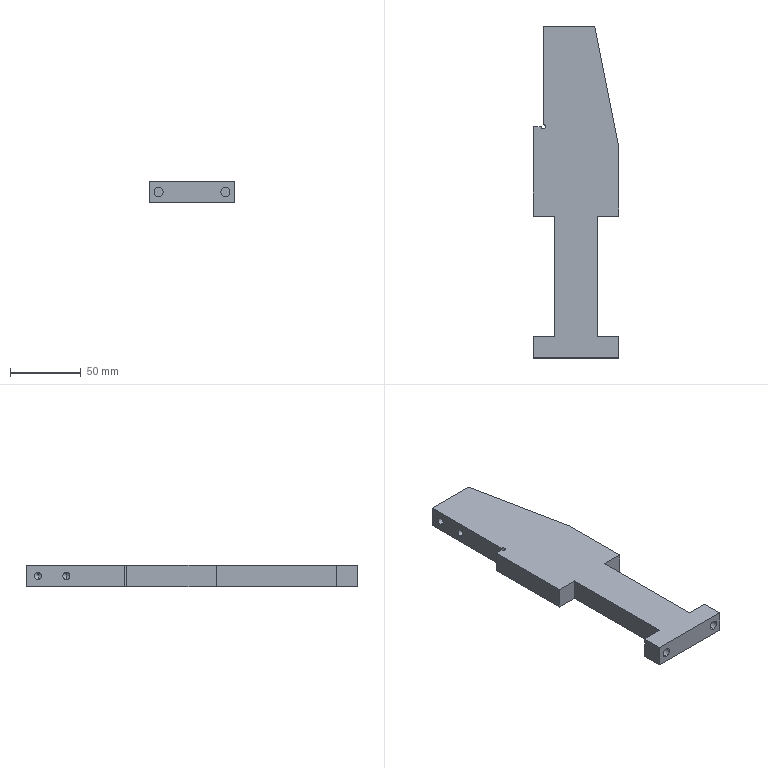Part | STEP file | 11-FG-E00211 | 1 solid | 31 faces | box 60 x 234 x 15 mm | volume 152627 mm3 | plane 17 | cylinder 10 | cone 4 | commonest cylinder face diameters 5 x4 6.5 x4 3 x2
STEP:
#1=CARTESIAN_POINT('',(6.5,0.,4.25));
#2=VERTEX_POINT('',#1);
#3=CARTESIAN_POINT('',(6.5,0.,10.75));
#4=VERTEX_POINT('',#3);
#5=CARTESIAN_POINT('',(6.5,0.,7.5));
#6=DIRECTION('',(0.,1.,0.));
#7=DIRECTION('',(0.,0.,1.));
#8=AXIS2_PLACEMENT_3D('',#5,#6,#7);
#9=CIRCLE('',#8,3.25);
#10=EDGE_CURVE('',#2,#4,#9,.T.);
#11=ORIENTED_EDGE('',*,*,#10,.F.);
#12=CARTESIAN_POINT('',(6.5,15.,4.25));
#13=VERTEX_POINT('',#12);
#14=CARTESIAN_POINT('',(6.5,-46.,4.25));
#15=DIRECTION('',(0.,1.,0.));
#16=VECTOR('',#15,1000.);
#17=LINE('',#14,#16);
#18=EDGE_CURVE('',#2,#13,#17,.T.);
#19=ORIENTED_EDGE('',*,*,#18,.T.);
#20=CARTESIAN_POINT('',(6.5,15.,10.75));
#21=VERTEX_POINT('',#20);
#22=CARTESIAN_POINT('',(6.5,15.,7.5));
#23=DIRECTION('',(0.,1.,0.));
#24=DIRECTION('',(0.,0.,1.));
#25=AXIS2_PLACEMENT_3D('',#22,#23,#24);
#26=CIRCLE('',#25,3.25);
#27=EDGE_CURVE('',#13,#21,#26,.T.);
#28=ORIENTED_EDGE('',*,*,#27,.T.);
#29=CARTESIAN_POINT('',(6.5,-46.,10.75));
#30=DIRECTION('',(0.,1.,0.));
#31=VECTOR('',#30,1000.);
#32=LINE('',#29,#31);
#33=EDGE_CURVE('',#4,#21,#32,.T.);
#34=ORIENTED_EDGE('',*,*,#33,.F.);
#35=EDGE_LOOP('',(#11,#19,#28,#34));
#36=FACE_OUTER_BOUND('',#35,.T.);
#37=CARTESIAN_POINT('',(6.5,-46.,7.5));
#38=DIRECTION('',(0.,1.,0.));
#39=DIRECTION('',(0.,0.,1.));
#40=AXIS2_PLACEMENT_3D('',#37,#38,#39);
#41=CYLINDRICAL_SURFACE('',#40,3.25);
#42=ADVANCED_FACE('',(#36),#41,.F.);
#43=CARTESIAN_POINT('',(53.5,0.,4.25));
#44=VERTEX_POINT('',#43);
#45=CARTESIAN_POINT('',(53.5,0.,10.75));
#46=VERTEX_POINT('',#45);
#47=CARTESIAN_POINT('',(53.5,0.,7.5));
#48=DIRECTION('',(0.,1.,0.));
#49=DIRECTION('',(0.,0.,1.));
#50=AXIS2_PLACEMENT_3D('',#47,#48,#49);
#51=CIRCLE('',#50,3.25);
#52=EDGE_CURVE('',#44,#46,#51,.T.);
#53=ORIENTED_EDGE('',*,*,#52,.F.);
#54=CARTESIAN_POINT('',(53.5,15.,4.25));
#55=VERTEX_POINT('',#54);
#56=CARTESIAN_POINT('',(53.5,-46.,4.25));
#57=DIRECTION('',(0.,1.,0.));
#58=VECTOR('',#57,1000.);
#59=LINE('',#56,#58);
#60=EDGE_CURVE('',#44,#55,#59,.T.);
#61=ORIENTED_EDGE('',*,*,#60,.T.);
#62=CARTESIAN_POINT('',(53.5,15.,10.75));
#63=VERTEX_POINT('',#62);
#64=CARTESIAN_POINT('',(53.5,15.,7.5));
#65=DIRECTION('',(0.,1.,0.));
#66=DIRECTION('',(0.,0.,1.));
#67=AXIS2_PLACEMENT_3D('',#64,#65,#66);
#68=CIRCLE('',#67,3.25);
#69=EDGE_CURVE('',#55,#63,#68,.T.);
#70=ORIENTED_EDGE('',*,*,#69,.T.);
#71=CARTESIAN_POINT('',(53.5,-46.,10.75));
#72=DIRECTION('',(0.,1.,0.));
#73=VECTOR('',#72,1000.);
#74=LINE('',#71,#73);
#75=EDGE_CURVE('',#46,#63,#74,.T.);
#76=ORIENTED_EDGE('',*,*,#75,.F.);
#77=EDGE_LOOP('',(#53,#61,#70,#76));
#78=FACE_OUTER_BOUND('',#77,.T.);
#79=CARTESIAN_POINT('',(53.5,-46.,7.5));
#80=DIRECTION('',(0.,1.,0.));
#81=DIRECTION('',(0.,0.,1.));
#82=AXIS2_PLACEMENT_3D('',#79,#80,#81);
#83=CYLINDRICAL_SURFACE('',#82,3.25);
#84=ADVANCED_FACE('',(#78),#83,.F.);
#85=CARTESIAN_POINT('',(23.502,205.5,7.5));
#86=VERTEX_POINT('',#85);
#87=CARTESIAN_POINT('',(22.,205.5,10.));
#88=VERTEX_POINT('',#87);
#89=CARTESIAN_POINT('',(22.,205.5,10.));
#90=DIRECTION('',(-0.515,0.,0.8572));
#91=VECTOR('',#90,1000.);
#92=LINE('',#89,#91);
#93=EDGE_CURVE('',#86,#88,#92,.T.);
#94=ORIENTED_EDGE('',*,*,#93,.F.);
#95=CARTESIAN_POINT('',(22.,205.5,5.));
#96=VERTEX_POINT('',#95);
#97=CARTESIAN_POINT('',(22.,205.5,5.));
#98=DIRECTION('',(-0.515,0.,-0.8572));
#99=VECTOR('',#98,1000.);
#100=LINE('',#97,#99);
#101=EDGE_CURVE('',#86,#96,#100,.T.);
#102=ORIENTED_EDGE('',*,*,#101,.T.);
#103=CARTESIAN_POINT('',(22.,205.5,7.5));
#104=DIRECTION('',(-1.,0.,0.));
#105=DIRECTION('',(0.,0.,1.));
#106=AXIS2_PLACEMENT_3D('',#103,#104,#105);
#107=CIRCLE('',#106,2.5);
#108=EDGE_CURVE('',#96,#88,#107,.T.);
#109=ORIENTED_EDGE('',*,*,#108,.T.);
#110=EDGE_LOOP('',(#94,#102,#109));
#111=FACE_OUTER_BOUND('',#110,.T.);
#112=CARTESIAN_POINT('',(22.,205.5,7.5));
#113=DIRECTION('',(-1.,0.,0.));
#114=DIRECTION('',(0.,0.,1.));
#115=AXIS2_PLACEMENT_3D('',#112,#113,#114);
#116=CONICAL_SURFACE('',#115,2.5,1.03);
#117=ADVANCED_FACE('',(#111),#116,.F.);
#118=ORIENTED_EDGE('',*,*,#108,.F.);
#119=CARTESIAN_POINT('',(7.,205.5,5.));
#120=VERTEX_POINT('',#119);
#121=CARTESIAN_POINT('',(7.,205.5,5.));
#122=DIRECTION('',(-1.,0.,0.));
#123=VECTOR('',#122,1000.);
#124=LINE('',#121,#123);
#125=EDGE_CURVE('',#96,#120,#124,.T.);
#126=ORIENTED_EDGE('',*,*,#125,.T.);
#127=CARTESIAN_POINT('',(7.,205.5,10.));
#128=VERTEX_POINT('',#127);
#129=CARTESIAN_POINT('',(7.,205.5,7.5));
#130=DIRECTION('',(-1.,0.,0.));
#131=DIRECTION('',(0.,0.,1.));
#132=AXIS2_PLACEMENT_3D('',#129,#130,#131);
#133=CIRCLE('',#132,2.5);
#134=EDGE_CURVE('',#120,#128,#133,.T.);
#135=ORIENTED_EDGE('',*,*,#134,.T.);
#136=CARTESIAN_POINT('',(7.,205.5,10.));
#137=DIRECTION('',(-1.,0.,0.));
#138=VECTOR('',#137,1000.);
#139=LINE('',#136,#138);
#140=EDGE_CURVE('',#88,#128,#139,.T.);
#141=ORIENTED_EDGE('',*,*,#140,.F.);
#142=EDGE_LOOP('',(#118,#126,#135,#141));
#143=FACE_OUTER_BOUND('',#142,.T.);
#144=CARTESIAN_POINT('',(7.,205.5,7.5));
#145=DIRECTION('',(-1.,0.,0.));
#146=DIRECTION('',(0.,0.,1.));
#147=AXIS2_PLACEMENT_3D('',#144,#145,#146);
#148=CYLINDRICAL_SURFACE('',#147,2.5);
#149=ADVANCED_FACE('',(#143),#148,.F.);
#150=CARTESIAN_POINT('',(23.502,225.5,7.5));
#151=VERTEX_POINT('',#150);
#152=CARTESIAN_POINT('',(22.,225.5,10.));
#153=VERTEX_POINT('',#152);
#154=CARTESIAN_POINT('',(22.,225.5,10.));
#155=DIRECTION('',(-0.515,0.,0.8572));
#156=VECTOR('',#155,1000.);
#157=LINE('',#154,#156);
#158=EDGE_CURVE('',#151,#153,#157,.T.);
#159=ORIENTED_EDGE('',*,*,#158,.F.);
#160=CARTESIAN_POINT('',(22.,225.5,5.));
#161=VERTEX_POINT('',#160);
#162=CARTESIAN_POINT('',(22.,225.5,5.));
#163=DIRECTION('',(-0.515,0.,-0.8572));
#164=VECTOR('',#163,1000.);
#165=LINE('',#162,#164);
#166=EDGE_CURVE('',#151,#161,#165,.T.);
#167=ORIENTED_EDGE('',*,*,#166,.T.);
#168=CARTESIAN_POINT('',(22.,225.5,7.5));
#169=DIRECTION('',(-1.,0.,0.));
#170=DIRECTION('',(0.,0.,1.));
#171=AXIS2_PLACEMENT_3D('',#168,#169,#170);
#172=CIRCLE('',#171,2.5);
#173=EDGE_CURVE('',#161,#153,#172,.T.);
#174=ORIENTED_EDGE('',*,*,#173,.T.);
#175=EDGE_LOOP('',(#159,#167,#174));
#176=FACE_OUTER_BOUND('',#175,.T.);
#177=CARTESIAN_POINT('',(22.,225.5,7.5));
#178=DIRECTION('',(-1.,0.,0.));
#179=DIRECTION('',(0.,0.,1.));
#180=AXIS2_PLACEMENT_3D('',#177,#178,#179);
#181=CONICAL_SURFACE('',#180,2.5,1.03);
#182=ADVANCED_FACE('',(#176),#181,.F.);
#183=ORIENTED_EDGE('',*,*,#173,.F.);
#184=CARTESIAN_POINT('',(7.,225.5,5.));
#185=VERTEX_POINT('',#184);
#186=CARTESIAN_POINT('',(7.,225.5,5.));
#187=DIRECTION('',(-1.,0.,0.));
#188=VECTOR('',#187,1000.);
#189=LINE('',#186,#188);
#190=EDGE_CURVE('',#161,#185,#189,.T.);
#191=ORIENTED_EDGE('',*,*,#190,.T.);
#192=CARTESIAN_POINT('',(7.,225.5,10.));
#193=VERTEX_POINT('',#192);
#194=CARTESIAN_POINT('',(7.,225.5,7.5));
#195=DIRECTION('',(-1.,0.,0.));
#196=DIRECTION('',(0.,0.,1.));
#197=AXIS2_PLACEMENT_3D('',#194,#195,#196);
#198=CIRCLE('',#197,2.5);
#199=EDGE_CURVE('',#185,#193,#198,.T.);
#200=ORIENTED_EDGE('',*,*,#199,.T.);
#201=CARTESIAN_POINT('',(7.,225.5,10.));
#202=DIRECTION('',(-1.,0.,0.));
#203=VECTOR('',#202,1000.);
#204=LINE('',#201,#203);
#205=EDGE_CURVE('',#153,#193,#204,.T.);
#206=ORIENTED_EDGE('',*,*,#205,.F.);
#207=EDGE_LOOP('',(#183,#191,#200,#206));
#208=FACE_OUTER_BOUND('',#207,.T.);
#209=CARTESIAN_POINT('',(7.,225.5,7.5));
#210=DIRECTION('',(-1.,0.,0.));
#211=DIRECTION('',(0.,0.,1.));
#212=AXIS2_PLACEMENT_3D('',#209,#210,#211);
#213=CYLINDRICAL_SURFACE('',#212,2.5);
#214=ADVANCED_FACE('',(#208),#213,.F.);
#215=CARTESIAN_POINT('',(8.5,163.,0.));
#216=VERTEX_POINT('',#215);
#217=CARTESIAN_POINT('',(7.,164.5,0.));
#218=VERTEX_POINT('',#217);
#219=CARTESIAN_POINT('',(7.,163.,0.));
#220=DIRECTION('',(0.,0.,1.));
#221=DIRECTION('',(1.,0.,0.));
#222=AXIS2_PLACEMENT_3D('',#219,#220,#221);
#223=CIRCLE('',#222,1.5);
#224=EDGE_CURVE('',#216,#218,#223,.T.);
#225=ORIENTED_EDGE('',*,*,#224,.F.);
#226=CARTESIAN_POINT('',(8.5,163.,15.));
#227=VERTEX_POINT('',#226);
#228=CARTESIAN_POINT('',(8.5,163.,0.));
#229=DIRECTION('',(0.,0.,1.));
#230=VECTOR('',#229,1000.);
#231=LINE('',#228,#230);
#232=EDGE_CURVE('',#216,#227,#231,.T.);
#233=ORIENTED_EDGE('',*,*,#232,.T.);
#234=CARTESIAN_POINT('',(7.,164.5,15.));
#235=VERTEX_POINT('',#234);
#236=CARTESIAN_POINT('',(7.,163.,15.));
#237=DIRECTION('',(0.,0.,1.));
#238=DIRECTION('',(1.,0.,0.));
#239=AXIS2_PLACEMENT_3D('',#236,#237,#238);
#240=CIRCLE('',#239,1.5);
#241=EDGE_CURVE('',#227,#235,#240,.T.);
#242=ORIENTED_EDGE('',*,*,#241,.T.);
#243=CARTESIAN_POINT('',(7.,164.5,0.));
#244=DIRECTION('',(0.,0.,1.));
#245=VECTOR('',#244,1000.);
#246=LINE('',#243,#245);
#247=EDGE_CURVE('',#218,#235,#246,.T.);
#248=ORIENTED_EDGE('',*,*,#247,.F.);
#249=EDGE_LOOP('',(#225,#233,#242,#248));
#250=FACE_OUTER_BOUND('',#249,.T.);
#251=CARTESIAN_POINT('',(7.,163.,0.));
#252=DIRECTION('',(0.,0.,1.));
#253=DIRECTION('',(1.,0.,0.));
#254=AXIS2_PLACEMENT_3D('',#251,#252,#253);
#255=CYLINDRICAL_SURFACE('',#254,1.5);
#256=ADVANCED_FACE('',(#250),#255,.F.);
#257=CARTESIAN_POINT('',(0.,15.,15.));
#258=VERTEX_POINT('',#257);
#259=CARTESIAN_POINT('',(0.,0.,15.));
#260=VERTEX_POINT('',#259);
#261=CARTESIAN_POINT('',(0.,0.,15.));
#262=DIRECTION('',(0.,-1.,0.));
#263=VECTOR('',#262,1000.);
#264=LINE('',#261,#263);
#265=EDGE_CURVE('',#258,#260,#264,.T.);
#266=ORIENTED_EDGE('',*,*,#265,.F.);
#267=CARTESIAN_POINT('',(0.,15.,0.));
#268=VERTEX_POINT('',#267);
#269=CARTESIAN_POINT('',(0.,15.,61.));
#270=DIRECTION('',(0.,0.,-1.));
#271=VECTOR('',#270,1000.);
#272=LINE('',#269,#271);
#273=EDGE_CURVE('',#258,#268,#272,.T.);
#274=ORIENTED_EDGE('',*,*,#273,.T.);
#275=CARTESIAN_POINT('',(0.,0.,0.));
#276=VERTEX_POINT('',#275);
#277=CARTESIAN_POINT('',(0.,0.,0.));
#278=DIRECTION('',(0.,-1.,0.));
#279=VECTOR('',#278,1000.);
#280=LINE('',#277,#279);
#281=EDGE_CURVE('',#268,#276,#280,.T.);
#282=ORIENTED_EDGE('',*,*,#281,.T.);
#283=CARTESIAN_POINT('',(0.,0.,15.));
#284=DIRECTION('',(0.,0.,-1.));
#285=VECTOR('',#284,1000.);
#286=LINE('',#283,#285);
#287=EDGE_CURVE('',#260,#276,#286,.T.);
#288=ORIENTED_EDGE('',*,*,#287,.F.);
#289=EDGE_LOOP('',(#266,#274,#282,#288));
#290=FACE_OUTER_BOUND('',#289,.T.);
#291=CARTESIAN_POINT('',(0.,0.,15.));
#292=DIRECTION('',(1.,0.,0.));
#293=DIRECTION('',(0.,0.,-1.));
#294=AXIS2_PLACEMENT_3D('',#291,#292,#293);
#295=PLANE('',#294);
#296=ADVANCED_FACE('',(#290),#295,.F.);
#297=CARTESIAN_POINT('',(60.,100.,15.));
#298=VERTEX_POINT('',#297);
#299=CARTESIAN_POINT('',(60.,150.,15.));
#300=VERTEX_POINT('',#299);
#301=CARTESIAN_POINT('',(60.,0.,15.));
#302=DIRECTION('',(0.,1.,0.));
#303=VECTOR('',#302,1000.);
#304=LINE('',#301,#303);
#305=EDGE_CURVE('',#298,#300,#304,.T.);
#306=ORIENTED_EDGE('',*,*,#305,.F.);
#307=CARTESIAN_POINT('',(60.,100.,0.));
#308=VERTEX_POINT('',#307);
#309=CARTESIAN_POINT('',(60.,100.,61.));
#310=DIRECTION('',(0.,0.,-1.));
#311=VECTOR('',#310,1000.);
#312=LINE('',#309,#311);
#313=EDGE_CURVE('',#298,#308,#312,.T.);
#314=ORIENTED_EDGE('',*,*,#313,.T.);
#315=CARTESIAN_POINT('',(60.,150.,0.));
#316=VERTEX_POINT('',#315);
#317=CARTESIAN_POINT('',(60.,0.,0.));
#318=DIRECTION('',(0.,1.,0.));
#319=VECTOR('',#318,1000.);
#320=LINE('',#317,#319);
#321=EDGE_CURVE('',#308,#316,#320,.T.);
#322=ORIENTED_EDGE('',*,*,#321,.T.);
#323=CARTESIAN_POINT('',(60.,150.,15.));
#324=DIRECTION('',(0.,0.,-1.));
#325=VECTOR('',#324,1000.);
#326=LINE('',#323,#325);
#327=EDGE_CURVE('',#300,#316,#326,.T.);
#328=ORIENTED_EDGE('',*,*,#327,.F.);
#329=EDGE_LOOP('',(#306,#314,#322,#328));
#330=FACE_OUTER_BOUND('',#329,.T.);
#331=CARTESIAN_POINT('',(60.,0.,15.));
#332=DIRECTION('',(-1.,0.,0.));
#333=DIRECTION('',(0.,0.,1.));
#334=AXIS2_PLACEMENT_3D('',#331,#332,#333);
#335=PLANE('',#334);
#336=ADVANCED_FACE('',(#330),#335,.F.);
#337=CARTESIAN_POINT('',(0.,163.,0.));
#338=VERTEX_POINT('',#337);
#339=CARTESIAN_POINT('',(0.,100.,0.));
#340=VERTEX_POINT('',#339);
#341=CARTESIAN_POINT('',(0.,0.,0.));
#342=DIRECTION('',(0.,-1.,0.));
#343=VECTOR('',#342,1000.);
#344=LINE('',#341,#343);
#345=EDGE_CURVE('',#338,#340,#344,.T.);
#346=ORIENTED_EDGE('',*,*,#345,.T.);
#347=CARTESIAN_POINT('',(0.,100.,15.));
#348=VERTEX_POINT('',#347);
#349=CARTESIAN_POINT('',(0.,100.,61.));
#350=DIRECTION('',(0.,0.,-1.));
#351=VECTOR('',#350,1000.);
#352=LINE('',#349,#351);
#353=EDGE_CURVE('',#348,#340,#352,.T.);
#354=ORIENTED_EDGE('',*,*,#353,.F.);
#355=CARTESIAN_POINT('',(0.,163.,15.));
#356=VERTEX_POINT('',#355);
#357=CARTESIAN_POINT('',(0.,0.,15.));
#358=DIRECTION('',(0.,-1.,0.));
#359=VECTOR('',#358,1000.);
#360=LINE('',#357,#359);
#361=EDGE_CURVE('',#356,#348,#360,.T.);
#362=ORIENTED_EDGE('',*,*,#361,.F.);
#363=CARTESIAN_POINT('',(0.,163.,0.));
#364=DIRECTION('',(0.,0.,1.));
#365=VECTOR('',#364,1000.);
#366=LINE('',#363,#365);
#367=EDGE_CURVE('',#338,#356,#366,.T.);
#368=ORIENTED_EDGE('',*,*,#367,.F.);
#369=EDGE_LOOP('',(#346,#354,#362,#368));
#370=FACE_OUTER_BOUND('',#369,.T.);
#371=CARTESIAN_POINT('',(0.,0.,15.));
#372=DIRECTION('',(1.,0.,0.));
#373=DIRECTION('',(0.,0.,-1.));
#374=AXIS2_PLACEMENT_3D('',#371,#372,#373);
#375=PLANE('',#374);
#376=ADVANCED_FACE('',(#370),#375,.F.);
#377=CARTESIAN_POINT('',(6.5,0.,7.5));
#378=DIRECTION('',(0.,1.,0.));
#379=DIRECTION('',(0.,0.,1.));
#380=AXIS2_PLACEMENT_3D('',#377,#378,#379);
#381=CIRCLE('',#380,3.25);
#382=EDGE_CURVE('',#4,#2,#381,.T.);
#383=ORIENTED_EDGE('',*,*,#382,.T.);
#384=ORIENTED_EDGE('',*,*,#10,.T.);
#385=EDGE_LOOP('',(#383,#384));
#386=FACE_BOUND('',#385,.T.);
#387=CARTESIAN_POINT('',(53.5,0.,7.5));
#388=DIRECTION('',(0.,1.,0.));
#389=DIRECTION('',(0.,0.,1.));
#390=AXIS2_PLACEMENT_3D('',#387,#388,#389);
#391=CIRCLE('',#390,3.25);
#392=EDGE_CURVE('',#46,#44,#391,.T.);
#393=ORIENTED_EDGE('',*,*,#392,.T.);
#394=ORIENTED_EDGE('',*,*,#52,.T.);
#395=EDGE_LOOP('',(#393,#394));
#396=FACE_BOUND('',#395,.T.);
#397=CARTESIAN_POINT('',(60.,0.,0.));
#398=VERTEX_POINT('',#397);
#399=CARTESIAN_POINT('',(0.,0.,0.));
#400=DIRECTION('',(1.,0.,0.));
#401=VECTOR('',#400,1000.);
#402=LINE('',#399,#401);
#403=EDGE_CURVE('',#276,#398,#402,.T.);
#404=ORIENTED_EDGE('',*,*,#403,.T.);
#405=CARTESIAN_POINT('',(60.,0.,15.));
#406=VERTEX_POINT('',#405);
#407=CARTESIAN_POINT('',(60.,0.,15.));
#408=DIRECTION('',(0.,0.,-1.));
#409=VECTOR('',#408,1000.);
#410=LINE('',#407,#409);
#411=EDGE_CURVE('',#406,#398,#410,.T.);
#412=ORIENTED_EDGE('',*,*,#411,.F.);
#413=CARTESIAN_POINT('',(0.,0.,15.));
#414=DIRECTION('',(1.,0.,0.));
#415=VECTOR('',#414,1000.);
#416=LINE('',#413,#415);
#417=EDGE_CURVE('',#260,#406,#416,.T.);
#418=ORIENTED_EDGE('',*,*,#417,.F.);
#419=ORIENTED_EDGE('',*,*,#287,.T.);
#420=EDGE_LOOP('',(#404,#412,#418,#419));
#421=FACE_OUTER_BOUND('',#420,.T.);
#422=CARTESIAN_POINT('',(0.,0.,15.));
#423=DIRECTION('',(0.,1.,0.));
#424=DIRECTION('',(0.,0.,1.));
#425=AXIS2_PLACEMENT_3D('',#422,#423,#424);
#426=PLANE('',#425);
#427=ADVANCED_FACE('',(#386,#396,#421),#426,.F.);
#428=CARTESIAN_POINT('',(60.,15.,0.));
#429=VERTEX_POINT('',#428);
#430=CARTESIAN_POINT('',(60.,0.,0.));
#431=DIRECTION('',(0.,1.,0.));
#432=VECTOR('',#431,1000.);
#433=LINE('',#430,#432);
#434=EDGE_CURVE('',#398,#429,#433,.T.);
#435=ORIENTED_EDGE('',*,*,#434,.T.);
#436=CARTESIAN_POINT('',(60.,15.,15.));
#437=VERTEX_POINT('',#436);
#438=CARTESIAN_POINT('',(60.,15.,61.));
#439=DIRECTION('',(0.,0.,-1.));
#440=VECTOR('',#439,1000.);
#441=LINE('',#438,#440);
#442=EDGE_CURVE('',#437,#429,#441,.T.);
#443=ORIENTED_EDGE('',*,*,#442,.F.);
#444=CARTESIAN_POINT('',(60.,0.,15.));
#445=DIRECTION('',(0.,1.,0.));
#446=VECTOR('',#445,1000.);
#447=LINE('',#444,#446);
#448=EDGE_CURVE('',#406,#437,#447,.T.);
#449=ORIENTED_EDGE('',*,*,#448,.F.);
#450=ORIENTED_EDGE('',*,*,#411,.T.);
#451=EDGE_LOOP('',(#435,#443,#449,#450));
#452=FACE_OUTER_BOUND('',#451,.T.);
#453=CARTESIAN_POINT('',(60.,0.,15.));
#454=DIRECTION('',(-1.,0.,0.));
#455=DIRECTION('',(0.,0.,1.));
#456=AXIS2_PLACEMENT_3D('',#453,#454,#455);
#457=PLANE('',#456);
#458=ADVANCED_FACE('',(#452),#457,.F.);
#459=CARTESIAN_POINT('',(43.2,234.,0.));
#460=VERTEX_POINT('',#459);
#461=CARTESIAN_POINT('',(40.,250.,0.));
#462=DIRECTION('',(-0.1961,0.9806,0.));
#463=VECTOR('',#462,1000.);
#464=LINE('',#461,#463);
#465=EDGE_CURVE('',#316,#460,#464,.T.);
#466=ORIENTED_EDGE('',*,*,#465,.T.);
#467=CARTESIAN_POINT('',(43.2,234.,15.));
#468=VERTEX_POINT('',#467);
#469=CARTESIAN_POINT('',(43.2,234.,15.));
#470=DIRECTION('',(0.,0.,1.));
#471=VECTOR('',#470,1000.);
#472=LINE('',#469,#471);
#473=EDGE_CURVE('',#460,#468,#472,.T.);
#474=ORIENTED_EDGE('',*,*,#473,.T.);
#475=CARTESIAN_POINT('',(40.,250.,15.));
#476=DIRECTION('',(-0.1961,0.9806,0.));
#477=VECTOR('',#476,1000.);
#478=LINE('',#475,#477);
#479=EDGE_CURVE('',#300,#468,#478,.T.);
#480=ORIENTED_EDGE('',*,*,#479,.F.);
#481=ORIENTED_EDGE('',*,*,#327,.T.);
#482=EDGE_LOOP('',(#466,#474,#480,#481));
#483=FACE_OUTER_BOUND('',#482,.T.);
#484=CARTESIAN_POINT('',(40.,250.,15.));
#485=DIRECTION('',(-0.9806,-0.1961,0.));
#486=DIRECTION('',(0.1961,-0.9806,0.));
#487=AXIS2_PLACEMENT_3D('',#484,#485,#486);
#488=PLANE('',#487);
#489=ADVANCED_FACE('',(#483),#488,.F.);
#490=ORIENTED_EDGE('',*,*,#479,.T.);
#491=CARTESIAN_POINT('',(7.,234.,15.));
#492=VERTEX_POINT('',#491);
#493=CARTESIAN_POINT('',(0.,234.,15.));
#494=DIRECTION('',(-1.,0.,0.));
#495=VECTOR('',#494,1000.);
#496=LINE('',#493,#495);
#497=EDGE_CURVE('',#468,#492,#496,.T.);
#498=ORIENTED_EDGE('',*,*,#497,.T.);
#499=CARTESIAN_POINT('',(7.,250.,15.));
#500=DIRECTION('',(0.,1.,0.));
#501=VECTOR('',#500,1000.);
#502=LINE('',#499,#501);
#503=EDGE_CURVE('',#235,#492,#502,.T.);
#504=ORIENTED_EDGE('',*,*,#503,.F.);
#505=ORIENTED_EDGE('',*,*,#241,.F.);
#506=CARTESIAN_POINT('',(5.5,163.,15.));
#507=VERTEX_POINT('',#506);
#508=CARTESIAN_POINT('',(7.,163.,15.));
#509=DIRECTION('',(0.,0.,1.));
#510=DIRECTION('',(1.,0.,0.));
#511=AXIS2_PLACEMENT_3D('',#508,#509,#510);
#512=CIRCLE('',#511,1.5);
#513=EDGE_CURVE('',#507,#227,#512,.T.);
#514=ORIENTED_EDGE('',*,*,#513,.F.);
#515=CARTESIAN_POINT('',(0.,163.,15.));
#516=DIRECTION('',(1.,0.,0.));
#517=VECTOR('',#516,1000.);
#518=LINE('',#515,#517);
#519=EDGE_CURVE('',#356,#507,#518,.T.);
#520=ORIENTED_EDGE('',*,*,#519,.F.);
#521=ORIENTED_EDGE('',*,*,#361,.T.);
#522=CARTESIAN_POINT('',(15.,100.,15.));
#523=VERTEX_POINT('',#522);
#524=CARTESIAN_POINT('',(0.,100.,15.));
#525=DIRECTION('',(1.,0.,0.));
#526=VECTOR('',#525,1000.);
#527=LINE('',#524,#526);
#528=EDGE_CURVE('',#348,#523,#527,.T.);
#529=ORIENTED_EDGE('',*,*,#528,.T.);
#530=CARTESIAN_POINT('',(15.,15.,15.));
#531=VERTEX_POINT('',#530);
#532=CARTESIAN_POINT('',(15.,250.,15.));
#533=DIRECTION('',(0.,-1.,0.));
#534=VECTOR('',#533,1000.);
#535=LINE('',#532,#534);
#536=EDGE_CURVE('',#523,#531,#535,.T.);
#537=ORIENTED_EDGE('',*,*,#536,.T.);
#538=CARTESIAN_POINT('',(0.,15.,15.));
#539=DIRECTION('',(-1.,0.,0.));
#540=VECTOR('',#539,1000.);
#541=LINE('',#538,#540);
#542=EDGE_CURVE('',#531,#258,#541,.T.);
#543=ORIENTED_EDGE('',*,*,#542,.T.);
#544=ORIENTED_EDGE('',*,*,#265,.T.);
#545=ORIENTED_EDGE('',*,*,#417,.T.);
#546=ORIENTED_EDGE('',*,*,#448,.T.);
#547=CARTESIAN_POINT('',(45.,15.,15.));
#548=VERTEX_POINT('',#547);
#549=CARTESIAN_POINT('',(0.,15.,15.));
#550=DIRECTION('',(-1.,0.,0.));
#551=VECTOR('',#550,1000.);
#552=LINE('',#549,#551);
#553=EDGE_CURVE('',#437,#548,#552,.T.);
#554=ORIENTED_EDGE('',*,*,#553,.T.);
#555=CARTESIAN_POINT('',(45.,100.,15.));
#556=VERTEX_POINT('',#555);
#557=CARTESIAN_POINT('',(45.,250.,15.));
#558=DIRECTION('',(0.,1.,0.));
#559=VECTOR('',#558,1000.);
#560=LINE('',#557,#559);
#561=EDGE_CURVE('',#548,#556,#560,.T.);
#562=ORIENTED_EDGE('',*,*,#561,.T.);
#563=CARTESIAN_POINT('',(0.,100.,15.));
#564=DIRECTION('',(1.,0.,0.));
#565=VECTOR('',#564,1000.);
#566=LINE('',#563,#565);
#567=EDGE_CURVE('',#556,#298,#566,.T.);
#568=ORIENTED_EDGE('',*,*,#567,.T.);
#569=ORIENTED_EDGE('',*,*,#305,.T.);
#570=EDGE_LOOP('',(#490,#498,#504,#505,#514,#520,#521,#529,#537,#543,#544,#545,#546,#554,#562,#568,#569));
#571=FACE_OUTER_BOUND('',#570,.T.);
#572=CARTESIAN_POINT('',(0.,250.,15.));
#573=DIRECTION('',(0.,0.,-1.));
#574=DIRECTION('',(-1.,0.,0.));
#575=AXIS2_PLACEMENT_3D('',#572,#573,#574);
#576=PLANE('',#575);
#577=ADVANCED_FACE('',(#571),#576,.F.);
#578=CARTESIAN_POINT('',(7.,234.,0.));
#579=VERTEX_POINT('',#578);
#580=CARTESIAN_POINT('',(7.,234.,0.));
#581=DIRECTION('',(-1.,0.,0.));
#582=VECTOR('',#581,1000.);
#583=LINE('',#580,#582);
#584=EDGE_CURVE('',#460,#579,#583,.T.);
#585=ORIENTED_EDGE('',*,*,#584,.F.);
#586=ORIENTED_EDGE('',*,*,#465,.F.);
#587=ORIENTED_EDGE('',*,*,#321,.F.);
#588=CARTESIAN_POINT('',(45.,100.,0.));
#589=VERTEX_POINT('',#588);
#590=CARTESIAN_POINT('',(60.,100.,0.));
#591=DIRECTION('',(1.,0.,0.));
#592=VECTOR('',#591,1000.);
#593=LINE('',#590,#592);
#594=EDGE_CURVE('',#589,#308,#593,.T.);
#595=ORIENTED_EDGE('',*,*,#594,.F.);
#596=CARTESIAN_POINT('',(45.,15.,0.));
#597=VERTEX_POINT('',#596);
#598=CARTESIAN_POINT('',(45.,100.,0.));
#599=DIRECTION('',(0.,1.,0.));
#600=VECTOR('',#599,1000.);
#601=LINE('',#598,#600);
#602=EDGE_CURVE('',#597,#589,#601,.T.);
#603=ORIENTED_EDGE('',*,*,#602,.F.);
#604=CARTESIAN_POINT('',(60.,15.,0.));
#605=DIRECTION('',(-1.,0.,0.));
#606=VECTOR('',#605,1000.);
#607=LINE('',#604,#606);
#608=EDGE_CURVE('',#429,#597,#607,.T.);
#609=ORIENTED_EDGE('',*,*,#608,.F.);
#610=ORIENTED_EDGE('',*,*,#434,.F.);
#611=ORIENTED_EDGE('',*,*,#403,.F.);
#612=ORIENTED_EDGE('',*,*,#281,.F.);
#613=CARTESIAN_POINT('',(15.,15.,0.));
#614=VERTEX_POINT('',#613);
#615=CARTESIAN_POINT('',(0.,15.,0.));
#616=DIRECTION('',(-1.,0.,0.));
#617=VECTOR('',#616,1000.);
#618=LINE('',#615,#617);
#619=EDGE_CURVE('',#614,#268,#618,.T.);
#620=ORIENTED_EDGE('',*,*,#619,.F.);
#621=CARTESIAN_POINT('',(15.,100.,0.));
#622=VERTEX_POINT('',#621);
#623=CARTESIAN_POINT('',(15.,100.,0.));
#624=DIRECTION('',(0.,-1.,0.));
#625=VECTOR('',#624,1000.);
#626=LINE('',#623,#625);
#627=EDGE_CURVE('',#622,#614,#626,.T.);
#628=ORIENTED_EDGE('',*,*,#627,.F.);
#629=CARTESIAN_POINT('',(0.,100.,0.));
#630=DIRECTION('',(1.,0.,0.));
#631=VECTOR('',#630,1000.);
#632=LINE('',#629,#631);
#633=EDGE_CURVE('',#340,#622,#632,.T.);
#634=ORIENTED_EDGE('',*,*,#633,.F.);
#635=ORIENTED_EDGE('',*,*,#345,.F.);
#636=CARTESIAN_POINT('',(5.5,163.,0.));
#637=VERTEX_POINT('',#636);
#638=CARTESIAN_POINT('',(0.,163.,0.));
#639=DIRECTION('',(1.,0.,0.));
#640=VECTOR('',#639,1000.);
#641=LINE('',#638,#640);
#642=EDGE_CURVE('',#338,#637,#641,.T.);
#643=ORIENTED_EDGE('',*,*,#642,.T.);
#644=CARTESIAN_POINT('',(7.,163.,0.));
#645=DIRECTION('',(0.,0.,1.));
#646=DIRECTION('',(1.,0.,0.));
#647=AXIS2_PLACEMENT_3D('',#644,#645,#646);
#648=CIRCLE('',#647,1.5);
#649=EDGE_CURVE('',#637,#216,#648,.T.);
#650=ORIENTED_EDGE('',*,*,#649,.T.);
#651=ORIENTED_EDGE('',*,*,#224,.T.);
#652=CARTESIAN_POINT('',(7.,250.,0.));
#653=DIRECTION('',(0.,1.,0.));
#654=VECTOR('',#653,1000.);
#655=LINE('',#652,#654);
#656=EDGE_CURVE('',#218,#579,#655,.T.);
#657=ORIENTED_EDGE('',*,*,#656,.T.);
#658=EDGE_LOOP('',(#585,#586,#587,#595,#603,#609,#610,#611,#612,#620,#628,#634,#635,#643,#650,#651,#657));
#659=FACE_OUTER_BOUND('',#658,.T.);
#660=CARTESIAN_POINT('',(0.,250.,0.));
#661=DIRECTION('',(0.,0.,-1.));
#662=DIRECTION('',(-1.,0.,0.));
#663=AXIS2_PLACEMENT_3D('',#660,#661,#662);
#664=PLANE('',#663);
#665=ADVANCED_FACE('',(#659),#664,.T.);
#666=CARTESIAN_POINT('',(7.,205.5,7.5));
#667=DIRECTION('',(-1.,0.,0.));
#668=DIRECTION('',(0.,0.,1.));
#669=AXIS2_PLACEMENT_3D('',#666,#667,#668);
#670=CIRCLE('',#669,2.5);
#671=EDGE_CURVE('',#128,#120,#670,.T.);
#672=ORIENTED_EDGE('',*,*,#671,.F.);
#673=ORIENTED_EDGE('',*,*,#134,.F.);
#674=EDGE_LOOP('',(#672,#673));
#675=FACE_BOUND('',#674,.T.);
#676=CARTESIAN_POINT('',(7.,225.5,7.5));
#677=DIRECTION('',(-1.,0.,0.));
#678=DIRECTION('',(0.,0.,1.));
#679=AXIS2_PLACEMENT_3D('',#676,#677,#678);
#680=CIRCLE('',#679,2.5);
#681=EDGE_CURVE('',#193,#185,#680,.T.);
#682=ORIENTED_EDGE('',*,*,#681,.F.);
#683=ORIENTED_EDGE('',*,*,#199,.F.);
#684=EDGE_LOOP('',(#682,#683));
#685=FACE_BOUND('',#684,.T.);
#686=ORIENTED_EDGE('',*,*,#503,.T.);
#687=CARTESIAN_POINT('',(7.,234.,0.));
#688=DIRECTION('',(0.,0.,-1.));
#689=VECTOR('',#688,1000.);
#690=LINE('',#687,#689);
#691=EDGE_CURVE('',#492,#579,#690,.T.);
#692=ORIENTED_EDGE('',*,*,#691,.T.);
#693=ORIENTED_EDGE('',*,*,#656,.F.);
#694=ORIENTED_EDGE('',*,*,#247,.T.);
#695=EDGE_LOOP('',(#686,#692,#693,#694));
#696=FACE_OUTER_BOUND('',#695,.T.);
#697=CARTESIAN_POINT('',(7.,250.,0.));
#698=DIRECTION('',(1.,0.,0.));
#699=DIRECTION('',(0.,1.,0.));
#700=AXIS2_PLACEMENT_3D('',#697,#698,#699);
#701=PLANE('',#700);
#702=ADVANCED_FACE('',(#675,#685,#696),#701,.F.);
#703=ORIENTED_EDGE('',*,*,#519,.T.);
#704=CARTESIAN_POINT('',(5.5,163.,0.));
#705=DIRECTION('',(0.,0.,-1.));
#706=VECTOR('',#705,1000.);
#707=LINE('',#704,#706);
#708=EDGE_CURVE('',#507,#637,#707,.T.);
#709=ORIENTED_EDGE('',*,*,#708,.T.);
#710=ORIENTED_EDGE('',*,*,#642,.F.);
#711=ORIENTED_EDGE('',*,*,#367,.T.);
#712=EDGE_LOOP('',(#703,#709,#710,#711));
#713=FACE_OUTER_BOUND('',#712,.T.);
#714=CARTESIAN_POINT('',(0.,163.,0.));
#715=DIRECTION('',(0.,-1.,0.));
#716=DIRECTION('',(0.,0.,-1.));
#717=AXIS2_PLACEMENT_3D('',#714,#715,#716);
#718=PLANE('',#717);
#719=ADVANCED_FACE('',(#713),#718,.F.);
#720=ORIENTED_EDGE('',*,*,#232,.F.);
#721=ORIENTED_EDGE('',*,*,#649,.F.);
#722=ORIENTED_EDGE('',*,*,#708,.F.);
#723=ORIENTED_EDGE('',*,*,#513,.T.);
#724=EDGE_LOOP('',(#720,#721,#722,#723));
#725=FACE_OUTER_BOUND('',#724,.T.);
#726=CARTESIAN_POINT('',(7.,163.,0.));
#727=DIRECTION('',(0.,0.,1.));
#728=DIRECTION('',(1.,0.,0.));
#729=AXIS2_PLACEMENT_3D('',#726,#727,#728);
#730=CYLINDRICAL_SURFACE('',#729,1.5);
#731=ADVANCED_FACE('',(#725),#730,.F.);
#732=ORIENTED_EDGE('',*,*,#190,.F.);
#733=CARTESIAN_POINT('',(22.,225.5,7.5));
#734=DIRECTION('',(-1.,0.,0.));
#735=DIRECTION('',(0.,0.,1.));
#736=AXIS2_PLACEMENT_3D('',#733,#734,#735);
#737=CIRCLE('',#736,2.5);
#738=EDGE_CURVE('',#153,#161,#737,.T.);
#739=ORIENTED_EDGE('',*,*,#738,.F.);
#740=ORIENTED_EDGE('',*,*,#205,.T.);
#741=ORIENTED_EDGE('',*,*,#681,.T.);
#742=EDGE_LOOP('',(#732,#739,#740,#741));
#743=FACE_OUTER_BOUND('',#742,.T.);
#744=CARTESIAN_POINT('',(7.,225.5,7.5));
#745=DIRECTION('',(-1.,0.,0.));
#746=DIRECTION('',(0.,0.,1.));
#747=AXIS2_PLACEMENT_3D('',#744,#745,#746);
#748=CYLINDRICAL_SURFACE('',#747,2.5);
#749=ADVANCED_FACE('',(#743),#748,.F.);
#750=ORIENTED_EDGE('',*,*,#166,.F.);
#751=ORIENTED_EDGE('',*,*,#158,.T.);
#752=ORIENTED_EDGE('',*,*,#738,.T.);
#753=EDGE_LOOP('',(#750,#751,#752));
#754=FACE_OUTER_BOUND('',#753,.T.);
#755=CARTESIAN_POINT('',(22.,225.5,7.5));
#756=DIRECTION('',(-1.,0.,0.));
#757=DIRECTION('',(0.,0.,1.));
#758=AXIS2_PLACEMENT_3D('',#755,#756,#757);
#759=CONICAL_SURFACE('',#758,2.5,1.03);
#760=ADVANCED_FACE('',(#754),#759,.F.);
#761=ORIENTED_EDGE('',*,*,#125,.F.);
#762=CARTESIAN_POINT('',(22.,205.5,7.5));
#763=DIRECTION('',(-1.,0.,0.));
#764=DIRECTION('',(0.,0.,1.));
#765=AXIS2_PLACEMENT_3D('',#762,#763,#764);
#766=CIRCLE('',#765,2.5);
#767=EDGE_CURVE('',#88,#96,#766,.T.);
#768=ORIENTED_EDGE('',*,*,#767,.F.);
#769=ORIENTED_EDGE('',*,*,#140,.T.);
#770=ORIENTED_EDGE('',*,*,#671,.T.);
#771=EDGE_LOOP('',(#761,#768,#769,#770));
#772=FACE_OUTER_BOUND('',#771,.T.);
#773=CARTESIAN_POINT('',(7.,205.5,7.5));
#774=DIRECTION('',(-1.,0.,0.));
#775=DIRECTION('',(0.,0.,1.));
#776=AXIS2_PLACEMENT_3D('',#773,#774,#775);
#777=CYLINDRICAL_SURFACE('',#776,2.5);
#778=ADVANCED_FACE('',(#772),#777,.F.);
#779=ORIENTED_EDGE('',*,*,#101,.F.);
#780=ORIENTED_EDGE('',*,*,#93,.T.);
#781=ORIENTED_EDGE('',*,*,#767,.T.);
#782=EDGE_LOOP('',(#779,#780,#781));
#783=FACE_OUTER_BOUND('',#782,.T.);
#784=CARTESIAN_POINT('',(22.,205.5,7.5));
#785=DIRECTION('',(-1.,0.,0.));
#786=DIRECTION('',(0.,0.,1.));
#787=AXIS2_PLACEMENT_3D('',#784,#785,#786);
#788=CONICAL_SURFACE('',#787,2.5,1.03);
#789=ADVANCED_FACE('',(#783),#788,.F.);
#790=CARTESIAN_POINT('',(45.,100.,61.));
#791=DIRECTION('',(0.,0.,-1.));
#792=VECTOR('',#791,1000.);
#793=LINE('',#790,#792);
#794=EDGE_CURVE('',#556,#589,#793,.T.);
#795=ORIENTED_EDGE('',*,*,#794,.T.);
#796=ORIENTED_EDGE('',*,*,#594,.T.);
#797=ORIENTED_EDGE('',*,*,#313,.F.);
#798=ORIENTED_EDGE('',*,*,#567,.F.);
#799=EDGE_LOOP('',(#795,#796,#797,#798));
#800=FACE_OUTER_BOUND('',#799,.T.);
#801=CARTESIAN_POINT('',(60.,100.,61.));
#802=DIRECTION('',(0.,1.,0.));
#803=DIRECTION('',(0.,0.,1.));
#804=AXIS2_PLACEMENT_3D('',#801,#802,#803);
#805=PLANE('',#804);
#806=ADVANCED_FACE('',(#800),#805,.F.);
#807=CARTESIAN_POINT('',(45.,15.,61.));
#808=DIRECTION('',(0.,0.,-1.));
#809=VECTOR('',#808,1000.);
#810=LINE('',#807,#809);
#811=EDGE_CURVE('',#548,#597,#810,.T.);
#812=ORIENTED_EDGE('',*,*,#811,.T.);
#813=ORIENTED_EDGE('',*,*,#602,.T.);
#814=ORIENTED_EDGE('',*,*,#794,.F.);
#815=ORIENTED_EDGE('',*,*,#561,.F.);
#816=EDGE_LOOP('',(#812,#813,#814,#815));
#817=FACE_OUTER_BOUND('',#816,.T.);
#818=CARTESIAN_POINT('',(45.,100.,61.));
#819=DIRECTION('',(-1.,0.,0.));
#820=DIRECTION('',(0.,-1.,0.));
#821=AXIS2_PLACEMENT_3D('',#818,#819,#820);
#822=PLANE('',#821);
#823=ADVANCED_FACE('',(#817),#822,.F.);
#824=CARTESIAN_POINT('',(53.5,15.,7.5));
#825=DIRECTION('',(0.,1.,0.));
#826=DIRECTION('',(0.,0.,1.));
#827=AXIS2_PLACEMENT_3D('',#824,#825,#826);
#828=CIRCLE('',#827,3.25);
#829=EDGE_CURVE('',#63,#55,#828,.T.);
#830=ORIENTED_EDGE('',*,*,#829,.F.);
#831=ORIENTED_EDGE('',*,*,#69,.F.);
#832=EDGE_LOOP('',(#830,#831));
#833=FACE_BOUND('',#832,.T.);
#834=ORIENTED_EDGE('',*,*,#442,.T.);
#835=ORIENTED_EDGE('',*,*,#608,.T.);
#836=ORIENTED_EDGE('',*,*,#811,.F.);
#837=ORIENTED_EDGE('',*,*,#553,.F.);
#838=EDGE_LOOP('',(#834,#835,#836,#837));
#839=FACE_OUTER_BOUND('',#838,.T.);
#840=CARTESIAN_POINT('',(60.,15.,61.));
#841=DIRECTION('',(0.,-1.,0.));
#842=DIRECTION('',(0.,0.,-1.));
#843=AXIS2_PLACEMENT_3D('',#840,#841,#842);
#844=PLANE('',#843);
#845=ADVANCED_FACE('',(#833,#839),#844,.F.);
#846=CARTESIAN_POINT('',(6.5,15.,7.5));
#847=DIRECTION('',(0.,1.,0.));
#848=DIRECTION('',(0.,0.,1.));
#849=AXIS2_PLACEMENT_3D('',#846,#847,#848);
#850=CIRCLE('',#849,3.25);
#851=EDGE_CURVE('',#21,#13,#850,.T.);
#852=ORIENTED_EDGE('',*,*,#851,.F.);
#853=ORIENTED_EDGE('',*,*,#27,.F.);
#854=EDGE_LOOP('',(#852,#853));
#855=FACE_BOUND('',#854,.T.);
#856=CARTESIAN_POINT('',(15.,15.,61.));
#857=DIRECTION('',(0.,0.,-1.));
#858=VECTOR('',#857,1000.);
#859=LINE('',#856,#858);
#860=EDGE_CURVE('',#531,#614,#859,.T.);
#861=ORIENTED_EDGE('',*,*,#860,.T.);
#862=ORIENTED_EDGE('',*,*,#619,.T.);
#863=ORIENTED_EDGE('',*,*,#273,.F.);
#864=ORIENTED_EDGE('',*,*,#542,.F.);
#865=EDGE_LOOP('',(#861,#862,#863,#864));
#866=FACE_OUTER_BOUND('',#865,.T.);
#867=CARTESIAN_POINT('',(0.,15.,61.));
#868=DIRECTION('',(0.,-1.,0.));
#869=DIRECTION('',(0.,0.,-1.));
#870=AXIS2_PLACEMENT_3D('',#867,#868,#869);
#871=PLANE('',#870);
#872=ADVANCED_FACE('',(#855,#866),#871,.F.);
#873=CARTESIAN_POINT('',(15.,100.,61.));
#874=DIRECTION('',(0.,0.,-1.));
#875=VECTOR('',#874,1000.);
#876=LINE('',#873,#875);
#877=EDGE_CURVE('',#523,#622,#876,.T.);
#878=ORIENTED_EDGE('',*,*,#877,.T.);
#879=ORIENTED_EDGE('',*,*,#627,.T.);
#880=ORIENTED_EDGE('',*,*,#860,.F.);
#881=ORIENTED_EDGE('',*,*,#536,.F.);
#882=EDGE_LOOP('',(#878,#879,#880,#881));
#883=FACE_OUTER_BOUND('',#882,.T.);
#884=CARTESIAN_POINT('',(15.,100.,61.));
#885=DIRECTION('',(1.,0.,0.));
#886=DIRECTION('',(0.,1.,0.));
#887=AXIS2_PLACEMENT_3D('',#884,#885,#886);
#888=PLANE('',#887);
#889=ADVANCED_FACE('',(#883),#888,.F.);
#890=ORIENTED_EDGE('',*,*,#353,.T.);
#891=ORIENTED_EDGE('',*,*,#633,.T.);
#892=ORIENTED_EDGE('',*,*,#877,.F.);
#893=ORIENTED_EDGE('',*,*,#528,.F.);
#894=EDGE_LOOP('',(#890,#891,#892,#893));
#895=FACE_OUTER_BOUND('',#894,.T.);
#896=CARTESIAN_POINT('',(0.,100.,61.));
#897=DIRECTION('',(0.,1.,0.));
#898=DIRECTION('',(0.,0.,1.));
#899=AXIS2_PLACEMENT_3D('',#896,#897,#898);
#900=PLANE('',#899);
#901=ADVANCED_FACE('',(#895),#900,.F.);
#902=ORIENTED_EDGE('',*,*,#60,.F.);
#903=ORIENTED_EDGE('',*,*,#392,.F.);
#904=ORIENTED_EDGE('',*,*,#75,.T.);
#905=ORIENTED_EDGE('',*,*,#829,.T.);
#906=EDGE_LOOP('',(#902,#903,#904,#905));
#907=FACE_OUTER_BOUND('',#906,.T.);
#908=CARTESIAN_POINT('',(53.5,-46.,7.5));
#909=DIRECTION('',(0.,1.,0.));
#910=DIRECTION('',(0.,0.,1.));
#911=AXIS2_PLACEMENT_3D('',#908,#909,#910);
#912=CYLINDRICAL_SURFACE('',#911,3.25);
#913=ADVANCED_FACE('',(#907),#912,.F.);
#914=ORIENTED_EDGE('',*,*,#18,.F.);
#915=ORIENTED_EDGE('',*,*,#382,.F.);
#916=ORIENTED_EDGE('',*,*,#33,.T.);
#917=ORIENTED_EDGE('',*,*,#851,.T.);
#918=EDGE_LOOP('',(#914,#915,#916,#917));
#919=FACE_OUTER_BOUND('',#918,.T.);
#920=CARTESIAN_POINT('',(6.5,-46.,7.5));
#921=DIRECTION('',(0.,1.,0.));
#922=DIRECTION('',(0.,0.,1.));
#923=AXIS2_PLACEMENT_3D('',#920,#921,#922);
#924=CYLINDRICAL_SURFACE('',#923,3.25);
#925=ADVANCED_FACE('',(#919),#924,.F.);
#926=ORIENTED_EDGE('',*,*,#584,.T.);
#927=ORIENTED_EDGE('',*,*,#691,.F.);
#928=ORIENTED_EDGE('',*,*,#497,.F.);
#929=ORIENTED_EDGE('',*,*,#473,.F.);
#930=EDGE_LOOP('',(#926,#927,#928,#929));
#931=FACE_OUTER_BOUND('',#930,.T.);
#932=CARTESIAN_POINT('',(7.,234.,31.));
#933=DIRECTION('',(0.,-1.,0.));
#934=DIRECTION('',(0.,0.,-1.));
#935=AXIS2_PLACEMENT_3D('',#932,#933,#934);
#936=PLANE('',#935);
#937=ADVANCED_FACE('',(#931),#936,.F.);
#938=CLOSED_SHELL('',(#42,#84,#117,#149,#182,#214,#256,#296,#336,#376,#427,#458,#489,#577,#665,#702,#719,#731,#749,#760,#778,#789,#806,#823,#845,#872,#889,#901,#913,#925,#937));
#939=MANIFOLD_SOLID_BREP('',#938);
#940=CARTESIAN_POINT('',(0.,0.,0.));
#941=DIRECTION('',(0.,0.,1.));
#942=DIRECTION('',(1.,0.,0.));
#943=AXIS2_PLACEMENT_3D('',#940,#941,#942);
#944=(LENGTH_UNIT()NAMED_UNIT(*)SI_UNIT(.MILLI.,.METRE.));
#945=UNCERTAINTY_MEASURE_WITH_UNIT(LENGTH_MEASURE(0.00001),#944,'','');
#946=(NAMED_UNIT(*)PLANE_ANGLE_UNIT()SI_UNIT($,.RADIAN.));
#947=(NAMED_UNIT(*)SI_UNIT($,.STERADIAN.)SOLID_ANGLE_UNIT());
#948=(GEOMETRIC_REPRESENTATION_CONTEXT(3)GLOBAL_UNCERTAINTY_ASSIGNED_CONTEXT((#945))GLOBAL_UNIT_ASSIGNED_CONTEXT((#944,#946,#947))REPRESENTATION_CONTEXT('',''));
#949=ADVANCED_BREP_SHAPE_REPRESENTATION('',(#939,#943),#948);